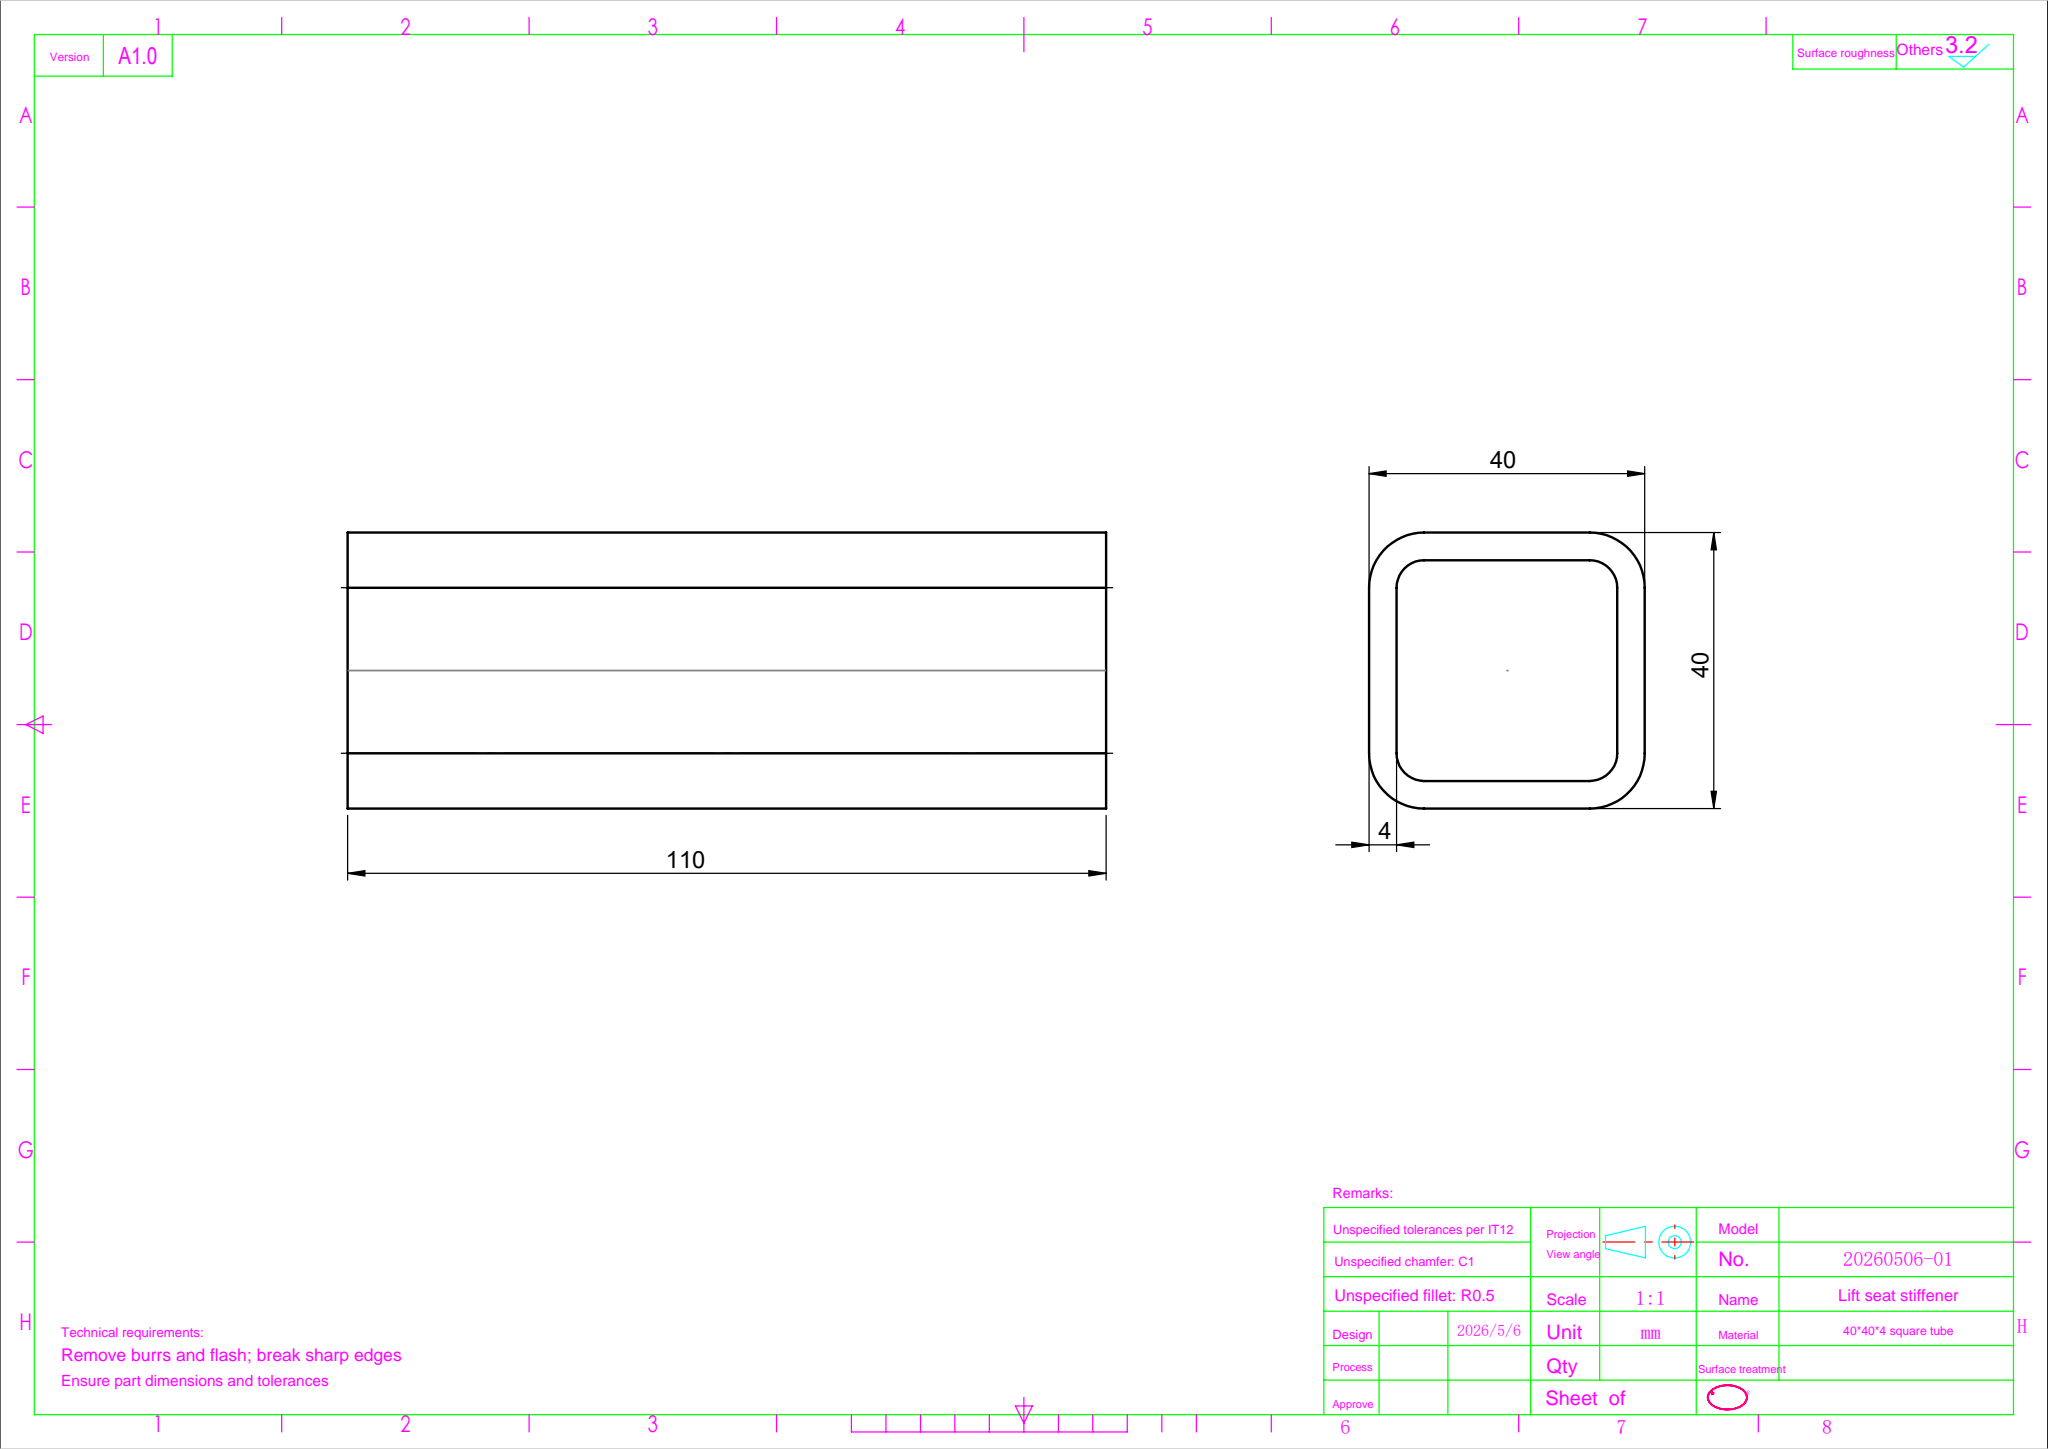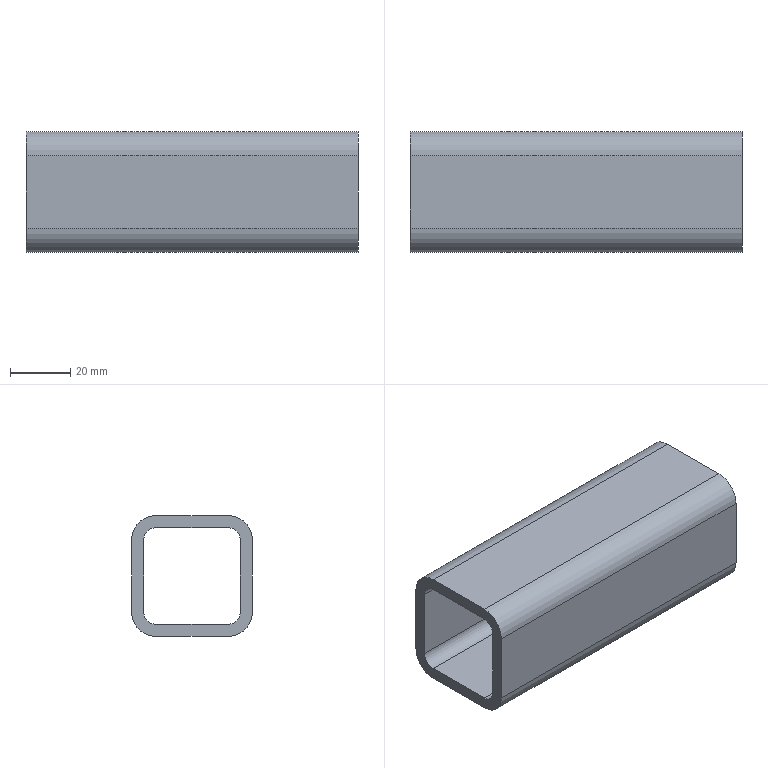Part | SolidWorks | features 3DProfileFeature 1, WeldMemberFeat 1, WeldmentFeature 1 | 1 solid | 18 faces | box 110 x 40 x 40 mm | volume 58828 mm3 | plane 10 | cylinder 8 | commonest cylinder face diameters 8 x4 16 x4
STEP:
#1=CARTESIAN_POINT('',(0.,12.,-20.));
#2=VERTEX_POINT('',#1);
#3=CARTESIAN_POINT('',(0.,20.,-12.));
#4=VERTEX_POINT('',#3);
#5=CARTESIAN_POINT('',(0.,12.,-12.));
#6=DIRECTION('',(1.,0.,0.));
#7=DIRECTION('',(0.,0.,-1.));
#8=AXIS2_PLACEMENT_3D('',#5,#6,#7);
#9=CIRCLE('',#8,8.);
#10=EDGE_CURVE('',#2,#4,#9,.T.);
#11=ORIENTED_EDGE('',*,*,#10,.T.);
#12=CARTESIAN_POINT('',(110.,20.,-12.));
#13=VERTEX_POINT('',#12);
#14=CARTESIAN_POINT('',(110.,20.,-12.));
#15=DIRECTION('',(-1.,0.,0.));
#16=VECTOR('',#15,1000.);
#17=LINE('',#14,#16);
#18=EDGE_CURVE('',#13,#4,#17,.T.);
#19=ORIENTED_EDGE('',*,*,#18,.F.);
#20=CARTESIAN_POINT('',(110.,12.,-20.));
#21=VERTEX_POINT('',#20);
#22=CARTESIAN_POINT('',(110.,12.,-12.));
#23=DIRECTION('',(1.,0.,0.));
#24=DIRECTION('',(0.,0.,-1.));
#25=AXIS2_PLACEMENT_3D('',#22,#23,#24);
#26=CIRCLE('',#25,8.);
#27=EDGE_CURVE('',#21,#13,#26,.T.);
#28=ORIENTED_EDGE('',*,*,#27,.F.);
#29=CARTESIAN_POINT('',(110.,12.,-20.));
#30=DIRECTION('',(-1.,0.,0.));
#31=VECTOR('',#30,1000.);
#32=LINE('',#29,#31);
#33=EDGE_CURVE('',#21,#2,#32,.T.);
#34=ORIENTED_EDGE('',*,*,#33,.T.);
#35=EDGE_LOOP('',(#11,#19,#28,#34));
#36=FACE_OUTER_BOUND('',#35,.T.);
#37=CARTESIAN_POINT('',(110.,12.,-12.));
#38=DIRECTION('',(-1.,0.,0.));
#39=DIRECTION('',(0.,0.,1.));
#40=AXIS2_PLACEMENT_3D('',#37,#38,#39);
#41=CYLINDRICAL_SURFACE('',#40,8.);
#42=ADVANCED_FACE('',(#36),#41,.T.);
#43=CARTESIAN_POINT('',(0.,20.,12.));
#44=VERTEX_POINT('',#43);
#45=CARTESIAN_POINT('',(0.,20.,-12.));
#46=DIRECTION('',(0.,0.,1.));
#47=VECTOR('',#46,1000.);
#48=LINE('',#45,#47);
#49=EDGE_CURVE('',#4,#44,#48,.T.);
#50=ORIENTED_EDGE('',*,*,#49,.T.);
#51=CARTESIAN_POINT('',(110.,20.,12.));
#52=VERTEX_POINT('',#51);
#53=CARTESIAN_POINT('',(110.,20.,12.));
#54=DIRECTION('',(-1.,0.,0.));
#55=VECTOR('',#54,1000.);
#56=LINE('',#53,#55);
#57=EDGE_CURVE('',#52,#44,#56,.T.);
#58=ORIENTED_EDGE('',*,*,#57,.F.);
#59=CARTESIAN_POINT('',(110.,20.,-12.));
#60=DIRECTION('',(0.,0.,1.));
#61=VECTOR('',#60,1000.);
#62=LINE('',#59,#61);
#63=EDGE_CURVE('',#13,#52,#62,.T.);
#64=ORIENTED_EDGE('',*,*,#63,.F.);
#65=ORIENTED_EDGE('',*,*,#18,.T.);
#66=EDGE_LOOP('',(#50,#58,#64,#65));
#67=FACE_OUTER_BOUND('',#66,.T.);
#68=CARTESIAN_POINT('',(110.,20.,-12.));
#69=DIRECTION('',(0.,-1.,0.));
#70=DIRECTION('',(0.,0.,-1.));
#71=AXIS2_PLACEMENT_3D('',#68,#69,#70);
#72=PLANE('',#71);
#73=ADVANCED_FACE('',(#67),#72,.F.);
#74=CARTESIAN_POINT('',(0.,12.,20.));
#75=VERTEX_POINT('',#74);
#76=CARTESIAN_POINT('',(0.,12.,12.));
#77=DIRECTION('',(1.,0.,0.));
#78=DIRECTION('',(0.,0.,-1.));
#79=AXIS2_PLACEMENT_3D('',#76,#77,#78);
#80=CIRCLE('',#79,8.);
#81=EDGE_CURVE('',#44,#75,#80,.T.);
#82=ORIENTED_EDGE('',*,*,#81,.T.);
#83=CARTESIAN_POINT('',(110.,12.,20.));
#84=VERTEX_POINT('',#83);
#85=CARTESIAN_POINT('',(110.,12.,20.));
#86=DIRECTION('',(-1.,0.,0.));
#87=VECTOR('',#86,1000.);
#88=LINE('',#85,#87);
#89=EDGE_CURVE('',#84,#75,#88,.T.);
#90=ORIENTED_EDGE('',*,*,#89,.F.);
#91=CARTESIAN_POINT('',(110.,12.,12.));
#92=DIRECTION('',(1.,0.,0.));
#93=DIRECTION('',(0.,0.,-1.));
#94=AXIS2_PLACEMENT_3D('',#91,#92,#93);
#95=CIRCLE('',#94,8.);
#96=EDGE_CURVE('',#52,#84,#95,.T.);
#97=ORIENTED_EDGE('',*,*,#96,.F.);
#98=ORIENTED_EDGE('',*,*,#57,.T.);
#99=EDGE_LOOP('',(#82,#90,#97,#98));
#100=FACE_OUTER_BOUND('',#99,.T.);
#101=CARTESIAN_POINT('',(110.,12.,12.));
#102=DIRECTION('',(-1.,0.,0.));
#103=DIRECTION('',(0.,0.,1.));
#104=AXIS2_PLACEMENT_3D('',#101,#102,#103);
#105=CYLINDRICAL_SURFACE('',#104,8.);
#106=ADVANCED_FACE('',(#100),#105,.T.);
#107=CARTESIAN_POINT('',(0.,-12.,20.));
#108=VERTEX_POINT('',#107);
#109=CARTESIAN_POINT('',(0.,-12.,20.));
#110=DIRECTION('',(0.,-1.,0.));
#111=VECTOR('',#110,1000.);
#112=LINE('',#109,#111);
#113=EDGE_CURVE('',#75,#108,#112,.T.);
#114=ORIENTED_EDGE('',*,*,#113,.T.);
#115=CARTESIAN_POINT('',(110.,-12.,20.));
#116=VERTEX_POINT('',#115);
#117=CARTESIAN_POINT('',(110.,-12.,20.));
#118=DIRECTION('',(-1.,0.,0.));
#119=VECTOR('',#118,1000.);
#120=LINE('',#117,#119);
#121=EDGE_CURVE('',#116,#108,#120,.T.);
#122=ORIENTED_EDGE('',*,*,#121,.F.);
#123=CARTESIAN_POINT('',(110.,-12.,20.));
#124=DIRECTION('',(0.,-1.,0.));
#125=VECTOR('',#124,1000.);
#126=LINE('',#123,#125);
#127=EDGE_CURVE('',#84,#116,#126,.T.);
#128=ORIENTED_EDGE('',*,*,#127,.F.);
#129=ORIENTED_EDGE('',*,*,#89,.T.);
#130=EDGE_LOOP('',(#114,#122,#128,#129));
#131=FACE_OUTER_BOUND('',#130,.T.);
#132=CARTESIAN_POINT('',(110.,-12.,20.));
#133=DIRECTION('',(0.,0.,-1.));
#134=DIRECTION('',(-1.,0.,0.));
#135=AXIS2_PLACEMENT_3D('',#132,#133,#134);
#136=PLANE('',#135);
#137=ADVANCED_FACE('',(#131),#136,.F.);
#138=CARTESIAN_POINT('',(0.,-20.,12.));
#139=VERTEX_POINT('',#138);
#140=CARTESIAN_POINT('',(0.,-12.,12.));
#141=DIRECTION('',(1.,0.,0.));
#142=DIRECTION('',(0.,0.,-1.));
#143=AXIS2_PLACEMENT_3D('',#140,#141,#142);
#144=CIRCLE('',#143,8.);
#145=EDGE_CURVE('',#108,#139,#144,.T.);
#146=ORIENTED_EDGE('',*,*,#145,.T.);
#147=CARTESIAN_POINT('',(110.,-20.,12.));
#148=VERTEX_POINT('',#147);
#149=CARTESIAN_POINT('',(110.,-20.,12.));
#150=DIRECTION('',(-1.,0.,0.));
#151=VECTOR('',#150,1000.);
#152=LINE('',#149,#151);
#153=EDGE_CURVE('',#148,#139,#152,.T.);
#154=ORIENTED_EDGE('',*,*,#153,.F.);
#155=CARTESIAN_POINT('',(110.,-12.,12.));
#156=DIRECTION('',(1.,0.,0.));
#157=DIRECTION('',(0.,0.,-1.));
#158=AXIS2_PLACEMENT_3D('',#155,#156,#157);
#159=CIRCLE('',#158,8.);
#160=EDGE_CURVE('',#116,#148,#159,.T.);
#161=ORIENTED_EDGE('',*,*,#160,.F.);
#162=ORIENTED_EDGE('',*,*,#121,.T.);
#163=EDGE_LOOP('',(#146,#154,#161,#162));
#164=FACE_OUTER_BOUND('',#163,.T.);
#165=CARTESIAN_POINT('',(110.,-12.,12.));
#166=DIRECTION('',(-1.,0.,0.));
#167=DIRECTION('',(0.,0.,1.));
#168=AXIS2_PLACEMENT_3D('',#165,#166,#167);
#169=CYLINDRICAL_SURFACE('',#168,8.);
#170=ADVANCED_FACE('',(#164),#169,.T.);
#171=CARTESIAN_POINT('',(0.,-20.,-12.));
#172=VERTEX_POINT('',#171);
#173=CARTESIAN_POINT('',(0.,-20.,12.));
#174=DIRECTION('',(0.,0.,-1.));
#175=VECTOR('',#174,1000.);
#176=LINE('',#173,#175);
#177=EDGE_CURVE('',#139,#172,#176,.T.);
#178=ORIENTED_EDGE('',*,*,#177,.T.);
#179=CARTESIAN_POINT('',(110.,-20.,-12.));
#180=VERTEX_POINT('',#179);
#181=CARTESIAN_POINT('',(110.,-20.,-12.));
#182=DIRECTION('',(-1.,0.,0.));
#183=VECTOR('',#182,1000.);
#184=LINE('',#181,#183);
#185=EDGE_CURVE('',#180,#172,#184,.T.);
#186=ORIENTED_EDGE('',*,*,#185,.F.);
#187=CARTESIAN_POINT('',(110.,-20.,12.));
#188=DIRECTION('',(0.,0.,-1.));
#189=VECTOR('',#188,1000.);
#190=LINE('',#187,#189);
#191=EDGE_CURVE('',#148,#180,#190,.T.);
#192=ORIENTED_EDGE('',*,*,#191,.F.);
#193=ORIENTED_EDGE('',*,*,#153,.T.);
#194=EDGE_LOOP('',(#178,#186,#192,#193));
#195=FACE_OUTER_BOUND('',#194,.T.);
#196=CARTESIAN_POINT('',(110.,-20.,12.));
#197=DIRECTION('',(0.,1.,0.));
#198=DIRECTION('',(0.,0.,1.));
#199=AXIS2_PLACEMENT_3D('',#196,#197,#198);
#200=PLANE('',#199);
#201=ADVANCED_FACE('',(#195),#200,.F.);
#202=CARTESIAN_POINT('',(0.,-12.,-20.));
#203=VERTEX_POINT('',#202);
#204=CARTESIAN_POINT('',(0.,-12.,-12.));
#205=DIRECTION('',(1.,0.,0.));
#206=DIRECTION('',(0.,0.,-1.));
#207=AXIS2_PLACEMENT_3D('',#204,#205,#206);
#208=CIRCLE('',#207,8.);
#209=EDGE_CURVE('',#172,#203,#208,.T.);
#210=ORIENTED_EDGE('',*,*,#209,.T.);
#211=CARTESIAN_POINT('',(110.,-12.,-20.));
#212=VERTEX_POINT('',#211);
#213=CARTESIAN_POINT('',(110.,-12.,-20.));
#214=DIRECTION('',(-1.,0.,0.));
#215=VECTOR('',#214,1000.);
#216=LINE('',#213,#215);
#217=EDGE_CURVE('',#212,#203,#216,.T.);
#218=ORIENTED_EDGE('',*,*,#217,.F.);
#219=CARTESIAN_POINT('',(110.,-12.,-12.));
#220=DIRECTION('',(1.,0.,0.));
#221=DIRECTION('',(0.,0.,-1.));
#222=AXIS2_PLACEMENT_3D('',#219,#220,#221);
#223=CIRCLE('',#222,8.);
#224=EDGE_CURVE('',#180,#212,#223,.T.);
#225=ORIENTED_EDGE('',*,*,#224,.F.);
#226=ORIENTED_EDGE('',*,*,#185,.T.);
#227=EDGE_LOOP('',(#210,#218,#225,#226));
#228=FACE_OUTER_BOUND('',#227,.T.);
#229=CARTESIAN_POINT('',(110.,-12.,-12.));
#230=DIRECTION('',(-1.,0.,0.));
#231=DIRECTION('',(0.,0.,1.));
#232=AXIS2_PLACEMENT_3D('',#229,#230,#231);
#233=CYLINDRICAL_SURFACE('',#232,8.);
#234=ADVANCED_FACE('',(#228),#233,.T.);
#235=CARTESIAN_POINT('',(0.,16.,12.));
#236=VERTEX_POINT('',#235);
#237=CARTESIAN_POINT('',(0.,12.,16.));
#238=VERTEX_POINT('',#237);
#239=CARTESIAN_POINT('',(0.,12.,12.));
#240=DIRECTION('',(1.,0.,0.));
#241=DIRECTION('',(0.,0.,-1.));
#242=AXIS2_PLACEMENT_3D('',#239,#240,#241);
#243=CIRCLE('',#242,4.);
#244=EDGE_CURVE('',#236,#238,#243,.T.);
#245=ORIENTED_EDGE('',*,*,#244,.F.);
#246=CARTESIAN_POINT('',(110.,16.,12.));
#247=VERTEX_POINT('',#246);
#248=CARTESIAN_POINT('',(110.,16.,12.));
#249=DIRECTION('',(-1.,0.,0.));
#250=VECTOR('',#249,1000.);
#251=LINE('',#248,#250);
#252=EDGE_CURVE('',#247,#236,#251,.T.);
#253=ORIENTED_EDGE('',*,*,#252,.F.);
#254=CARTESIAN_POINT('',(110.,12.,16.));
#255=VERTEX_POINT('',#254);
#256=CARTESIAN_POINT('',(110.,12.,12.));
#257=DIRECTION('',(1.,0.,0.));
#258=DIRECTION('',(0.,0.,-1.));
#259=AXIS2_PLACEMENT_3D('',#256,#257,#258);
#260=CIRCLE('',#259,4.);
#261=EDGE_CURVE('',#247,#255,#260,.T.);
#262=ORIENTED_EDGE('',*,*,#261,.T.);
#263=CARTESIAN_POINT('',(110.,12.,16.));
#264=DIRECTION('',(-1.,0.,0.));
#265=VECTOR('',#264,1000.);
#266=LINE('',#263,#265);
#267=EDGE_CURVE('',#255,#238,#266,.T.);
#268=ORIENTED_EDGE('',*,*,#267,.T.);
#269=EDGE_LOOP('',(#245,#253,#262,#268));
#270=FACE_OUTER_BOUND('',#269,.T.);
#271=CARTESIAN_POINT('',(110.,12.,12.));
#272=DIRECTION('',(-1.,0.,0.));
#273=DIRECTION('',(0.,0.,1.));
#274=AXIS2_PLACEMENT_3D('',#271,#272,#273);
#275=CYLINDRICAL_SURFACE('',#274,4.);
#276=ADVANCED_FACE('',(#270),#275,.F.);
#277=CARTESIAN_POINT('',(0.,16.,-12.));
#278=VERTEX_POINT('',#277);
#279=CARTESIAN_POINT('',(0.,16.,-12.));
#280=DIRECTION('',(0.,0.,1.));
#281=VECTOR('',#280,1000.);
#282=LINE('',#279,#281);
#283=EDGE_CURVE('',#278,#236,#282,.T.);
#284=ORIENTED_EDGE('',*,*,#283,.F.);
#285=CARTESIAN_POINT('',(110.,16.,-12.));
#286=VERTEX_POINT('',#285);
#287=CARTESIAN_POINT('',(110.,16.,-12.));
#288=DIRECTION('',(-1.,0.,0.));
#289=VECTOR('',#288,1000.);
#290=LINE('',#287,#289);
#291=EDGE_CURVE('',#286,#278,#290,.T.);
#292=ORIENTED_EDGE('',*,*,#291,.F.);
#293=CARTESIAN_POINT('',(110.,16.,-12.));
#294=DIRECTION('',(0.,0.,1.));
#295=VECTOR('',#294,1000.);
#296=LINE('',#293,#295);
#297=EDGE_CURVE('',#286,#247,#296,.T.);
#298=ORIENTED_EDGE('',*,*,#297,.T.);
#299=ORIENTED_EDGE('',*,*,#252,.T.);
#300=EDGE_LOOP('',(#284,#292,#298,#299));
#301=FACE_OUTER_BOUND('',#300,.T.);
#302=CARTESIAN_POINT('',(110.,16.,-12.));
#303=DIRECTION('',(0.,-1.,0.));
#304=DIRECTION('',(0.,0.,-1.));
#305=AXIS2_PLACEMENT_3D('',#302,#303,#304);
#306=PLANE('',#305);
#307=ADVANCED_FACE('',(#301),#306,.T.);
#308=CARTESIAN_POINT('',(0.,12.,-16.));
#309=VERTEX_POINT('',#308);
#310=CARTESIAN_POINT('',(0.,12.,-12.));
#311=DIRECTION('',(1.,0.,0.));
#312=DIRECTION('',(0.,0.,-1.));
#313=AXIS2_PLACEMENT_3D('',#310,#311,#312);
#314=CIRCLE('',#313,4.);
#315=EDGE_CURVE('',#309,#278,#314,.T.);
#316=ORIENTED_EDGE('',*,*,#315,.F.);
#317=CARTESIAN_POINT('',(110.,12.,-16.));
#318=VERTEX_POINT('',#317);
#319=CARTESIAN_POINT('',(110.,12.,-16.));
#320=DIRECTION('',(-1.,0.,0.));
#321=VECTOR('',#320,1000.);
#322=LINE('',#319,#321);
#323=EDGE_CURVE('',#318,#309,#322,.T.);
#324=ORIENTED_EDGE('',*,*,#323,.F.);
#325=CARTESIAN_POINT('',(110.,12.,-12.));
#326=DIRECTION('',(1.,0.,0.));
#327=DIRECTION('',(0.,0.,-1.));
#328=AXIS2_PLACEMENT_3D('',#325,#326,#327);
#329=CIRCLE('',#328,4.);
#330=EDGE_CURVE('',#318,#286,#329,.T.);
#331=ORIENTED_EDGE('',*,*,#330,.T.);
#332=ORIENTED_EDGE('',*,*,#291,.T.);
#333=EDGE_LOOP('',(#316,#324,#331,#332));
#334=FACE_OUTER_BOUND('',#333,.T.);
#335=CARTESIAN_POINT('',(110.,12.,-12.));
#336=DIRECTION('',(-1.,0.,0.));
#337=DIRECTION('',(0.,0.,1.));
#338=AXIS2_PLACEMENT_3D('',#335,#336,#337);
#339=CYLINDRICAL_SURFACE('',#338,4.);
#340=ADVANCED_FACE('',(#334),#339,.F.);
#341=CARTESIAN_POINT('',(0.,-12.,-16.));
#342=VERTEX_POINT('',#341);
#343=CARTESIAN_POINT('',(0.,12.,-16.));
#344=DIRECTION('',(0.,1.,0.));
#345=VECTOR('',#344,1000.);
#346=LINE('',#343,#345);
#347=EDGE_CURVE('',#342,#309,#346,.T.);
#348=ORIENTED_EDGE('',*,*,#347,.F.);
#349=CARTESIAN_POINT('',(110.,-12.,-16.));
#350=VERTEX_POINT('',#349);
#351=CARTESIAN_POINT('',(110.,-12.,-16.));
#352=DIRECTION('',(-1.,0.,0.));
#353=VECTOR('',#352,1000.);
#354=LINE('',#351,#353);
#355=EDGE_CURVE('',#350,#342,#354,.T.);
#356=ORIENTED_EDGE('',*,*,#355,.F.);
#357=CARTESIAN_POINT('',(110.,12.,-16.));
#358=DIRECTION('',(0.,1.,0.));
#359=VECTOR('',#358,1000.);
#360=LINE('',#357,#359);
#361=EDGE_CURVE('',#350,#318,#360,.T.);
#362=ORIENTED_EDGE('',*,*,#361,.T.);
#363=ORIENTED_EDGE('',*,*,#323,.T.);
#364=EDGE_LOOP('',(#348,#356,#362,#363));
#365=FACE_OUTER_BOUND('',#364,.T.);
#366=CARTESIAN_POINT('',(110.,12.,-16.));
#367=DIRECTION('',(0.,0.,1.));
#368=DIRECTION('',(1.,0.,0.));
#369=AXIS2_PLACEMENT_3D('',#366,#367,#368);
#370=PLANE('',#369);
#371=ADVANCED_FACE('',(#365),#370,.T.);
#372=CARTESIAN_POINT('',(0.,-16.,-12.));
#373=VERTEX_POINT('',#372);
#374=CARTESIAN_POINT('',(0.,-12.,-12.));
#375=DIRECTION('',(1.,0.,0.));
#376=DIRECTION('',(0.,0.,-1.));
#377=AXIS2_PLACEMENT_3D('',#374,#375,#376);
#378=CIRCLE('',#377,4.);
#379=EDGE_CURVE('',#373,#342,#378,.T.);
#380=ORIENTED_EDGE('',*,*,#379,.F.);
#381=CARTESIAN_POINT('',(110.,-16.,-12.));
#382=VERTEX_POINT('',#381);
#383=CARTESIAN_POINT('',(110.,-16.,-12.));
#384=DIRECTION('',(-1.,0.,0.));
#385=VECTOR('',#384,1000.);
#386=LINE('',#383,#385);
#387=EDGE_CURVE('',#382,#373,#386,.T.);
#388=ORIENTED_EDGE('',*,*,#387,.F.);
#389=CARTESIAN_POINT('',(110.,-12.,-12.));
#390=DIRECTION('',(1.,0.,0.));
#391=DIRECTION('',(0.,0.,-1.));
#392=AXIS2_PLACEMENT_3D('',#389,#390,#391);
#393=CIRCLE('',#392,4.);
#394=EDGE_CURVE('',#382,#350,#393,.T.);
#395=ORIENTED_EDGE('',*,*,#394,.T.);
#396=ORIENTED_EDGE('',*,*,#355,.T.);
#397=EDGE_LOOP('',(#380,#388,#395,#396));
#398=FACE_OUTER_BOUND('',#397,.T.);
#399=CARTESIAN_POINT('',(110.,-12.,-12.));
#400=DIRECTION('',(-1.,0.,0.));
#401=DIRECTION('',(0.,0.,1.));
#402=AXIS2_PLACEMENT_3D('',#399,#400,#401);
#403=CYLINDRICAL_SURFACE('',#402,4.);
#404=ADVANCED_FACE('',(#398),#403,.F.);
#405=CARTESIAN_POINT('',(0.,-16.,12.));
#406=VERTEX_POINT('',#405);
#407=CARTESIAN_POINT('',(0.,-16.,12.));
#408=DIRECTION('',(0.,0.,-1.));
#409=VECTOR('',#408,1000.);
#410=LINE('',#407,#409);
#411=EDGE_CURVE('',#406,#373,#410,.T.);
#412=ORIENTED_EDGE('',*,*,#411,.F.);
#413=CARTESIAN_POINT('',(110.,-16.,12.));
#414=VERTEX_POINT('',#413);
#415=CARTESIAN_POINT('',(110.,-16.,12.));
#416=DIRECTION('',(-1.,0.,0.));
#417=VECTOR('',#416,1000.);
#418=LINE('',#415,#417);
#419=EDGE_CURVE('',#414,#406,#418,.T.);
#420=ORIENTED_EDGE('',*,*,#419,.F.);
#421=CARTESIAN_POINT('',(110.,-16.,12.));
#422=DIRECTION('',(0.,0.,-1.));
#423=VECTOR('',#422,1000.);
#424=LINE('',#421,#423);
#425=EDGE_CURVE('',#414,#382,#424,.T.);
#426=ORIENTED_EDGE('',*,*,#425,.T.);
#427=ORIENTED_EDGE('',*,*,#387,.T.);
#428=EDGE_LOOP('',(#412,#420,#426,#427));
#429=FACE_OUTER_BOUND('',#428,.T.);
#430=CARTESIAN_POINT('',(110.,-16.,12.));
#431=DIRECTION('',(0.,1.,0.));
#432=DIRECTION('',(0.,0.,1.));
#433=AXIS2_PLACEMENT_3D('',#430,#431,#432);
#434=PLANE('',#433);
#435=ADVANCED_FACE('',(#429),#434,.T.);
#436=CARTESIAN_POINT('',(0.,-12.,16.));
#437=VERTEX_POINT('',#436);
#438=CARTESIAN_POINT('',(0.,-12.,12.));
#439=DIRECTION('',(1.,0.,0.));
#440=DIRECTION('',(0.,0.,-1.));
#441=AXIS2_PLACEMENT_3D('',#438,#439,#440);
#442=CIRCLE('',#441,4.);
#443=EDGE_CURVE('',#437,#406,#442,.T.);
#444=ORIENTED_EDGE('',*,*,#443,.F.);
#445=CARTESIAN_POINT('',(110.,-12.,16.));
#446=VERTEX_POINT('',#445);
#447=CARTESIAN_POINT('',(110.,-12.,16.));
#448=DIRECTION('',(-1.,0.,0.));
#449=VECTOR('',#448,1000.);
#450=LINE('',#447,#449);
#451=EDGE_CURVE('',#446,#437,#450,.T.);
#452=ORIENTED_EDGE('',*,*,#451,.F.);
#453=CARTESIAN_POINT('',(110.,-12.,12.));
#454=DIRECTION('',(1.,0.,0.));
#455=DIRECTION('',(0.,0.,-1.));
#456=AXIS2_PLACEMENT_3D('',#453,#454,#455);
#457=CIRCLE('',#456,4.);
#458=EDGE_CURVE('',#446,#414,#457,.T.);
#459=ORIENTED_EDGE('',*,*,#458,.T.);
#460=ORIENTED_EDGE('',*,*,#419,.T.);
#461=EDGE_LOOP('',(#444,#452,#459,#460));
#462=FACE_OUTER_BOUND('',#461,.T.);
#463=CARTESIAN_POINT('',(110.,-12.,12.));
#464=DIRECTION('',(-1.,0.,0.));
#465=DIRECTION('',(0.,0.,1.));
#466=AXIS2_PLACEMENT_3D('',#463,#464,#465);
#467=CYLINDRICAL_SURFACE('',#466,4.);
#468=ADVANCED_FACE('',(#462),#467,.F.);
#469=CARTESIAN_POINT('',(0.,-12.,16.));
#470=DIRECTION('',(0.,-1.,0.));
#471=VECTOR('',#470,1000.);
#472=LINE('',#469,#471);
#473=EDGE_CURVE('',#238,#437,#472,.T.);
#474=ORIENTED_EDGE('',*,*,#473,.F.);
#475=ORIENTED_EDGE('',*,*,#267,.F.);
#476=CARTESIAN_POINT('',(110.,-12.,16.));
#477=DIRECTION('',(0.,-1.,0.));
#478=VECTOR('',#477,1000.);
#479=LINE('',#476,#478);
#480=EDGE_CURVE('',#255,#446,#479,.T.);
#481=ORIENTED_EDGE('',*,*,#480,.T.);
#482=ORIENTED_EDGE('',*,*,#451,.T.);
#483=EDGE_LOOP('',(#474,#475,#481,#482));
#484=FACE_OUTER_BOUND('',#483,.T.);
#485=CARTESIAN_POINT('',(110.,-12.,16.));
#486=DIRECTION('',(0.,0.,-1.));
#487=DIRECTION('',(-1.,0.,0.));
#488=AXIS2_PLACEMENT_3D('',#485,#486,#487);
#489=PLANE('',#488);
#490=ADVANCED_FACE('',(#484),#489,.T.);
#491=CARTESIAN_POINT('',(0.,12.,-20.));
#492=DIRECTION('',(0.,1.,0.));
#493=VECTOR('',#492,1000.);
#494=LINE('',#491,#493);
#495=EDGE_CURVE('',#203,#2,#494,.T.);
#496=ORIENTED_EDGE('',*,*,#495,.T.);
#497=ORIENTED_EDGE('',*,*,#33,.F.);
#498=CARTESIAN_POINT('',(110.,12.,-20.));
#499=DIRECTION('',(0.,1.,0.));
#500=VECTOR('',#499,1000.);
#501=LINE('',#498,#500);
#502=EDGE_CURVE('',#212,#21,#501,.T.);
#503=ORIENTED_EDGE('',*,*,#502,.F.);
#504=ORIENTED_EDGE('',*,*,#217,.T.);
#505=EDGE_LOOP('',(#496,#497,#503,#504));
#506=FACE_OUTER_BOUND('',#505,.T.);
#507=CARTESIAN_POINT('',(110.,12.,-20.));
#508=DIRECTION('',(0.,0.,1.));
#509=DIRECTION('',(1.,0.,0.));
#510=AXIS2_PLACEMENT_3D('',#507,#508,#509);
#511=PLANE('',#510);
#512=ADVANCED_FACE('',(#506),#511,.F.);
#513=ORIENTED_EDGE('',*,*,#261,.F.);
#514=ORIENTED_EDGE('',*,*,#297,.F.);
#515=ORIENTED_EDGE('',*,*,#330,.F.);
#516=ORIENTED_EDGE('',*,*,#361,.F.);
#517=ORIENTED_EDGE('',*,*,#394,.F.);
#518=ORIENTED_EDGE('',*,*,#425,.F.);
#519=ORIENTED_EDGE('',*,*,#458,.F.);
#520=ORIENTED_EDGE('',*,*,#480,.F.);
#521=EDGE_LOOP('',(#513,#514,#515,#516,#517,#518,#519,#520));
#522=FACE_BOUND('',#521,.T.);
#523=ORIENTED_EDGE('',*,*,#27,.T.);
#524=ORIENTED_EDGE('',*,*,#63,.T.);
#525=ORIENTED_EDGE('',*,*,#96,.T.);
#526=ORIENTED_EDGE('',*,*,#127,.T.);
#527=ORIENTED_EDGE('',*,*,#160,.T.);
#528=ORIENTED_EDGE('',*,*,#191,.T.);
#529=ORIENTED_EDGE('',*,*,#224,.T.);
#530=ORIENTED_EDGE('',*,*,#502,.T.);
#531=EDGE_LOOP('',(#523,#524,#525,#526,#527,#528,#529,#530));
#532=FACE_OUTER_BOUND('',#531,.T.);
#533=CARTESIAN_POINT('',(110.,12.,-12.));
#534=DIRECTION('',(1.,0.,0.));
#535=DIRECTION('',(0.,0.,-1.));
#536=AXIS2_PLACEMENT_3D('',#533,#534,#535);
#537=PLANE('',#536);
#538=ADVANCED_FACE('',(#522,#532),#537,.T.);
#539=ORIENTED_EDGE('',*,*,#244,.T.);
#540=ORIENTED_EDGE('',*,*,#473,.T.);
#541=ORIENTED_EDGE('',*,*,#443,.T.);
#542=ORIENTED_EDGE('',*,*,#411,.T.);
#543=ORIENTED_EDGE('',*,*,#379,.T.);
#544=ORIENTED_EDGE('',*,*,#347,.T.);
#545=ORIENTED_EDGE('',*,*,#315,.T.);
#546=ORIENTED_EDGE('',*,*,#283,.T.);
#547=EDGE_LOOP('',(#539,#540,#541,#542,#543,#544,#545,#546));
#548=FACE_BOUND('',#547,.T.);
#549=ORIENTED_EDGE('',*,*,#10,.F.);
#550=ORIENTED_EDGE('',*,*,#495,.F.);
#551=ORIENTED_EDGE('',*,*,#209,.F.);
#552=ORIENTED_EDGE('',*,*,#177,.F.);
#553=ORIENTED_EDGE('',*,*,#145,.F.);
#554=ORIENTED_EDGE('',*,*,#113,.F.);
#555=ORIENTED_EDGE('',*,*,#81,.F.);
#556=ORIENTED_EDGE('',*,*,#49,.F.);
#557=EDGE_LOOP('',(#549,#550,#551,#552,#553,#554,#555,#556));
#558=FACE_OUTER_BOUND('',#557,.T.);
#559=CARTESIAN_POINT('',(0.,12.,-12.));
#560=DIRECTION('',(1.,0.,0.));
#561=DIRECTION('',(0.,0.,-1.));
#562=AXIS2_PLACEMENT_3D('',#559,#560,#561);
#563=PLANE('',#562);
#564=ADVANCED_FACE('',(#548,#558),#563,.F.);
#565=CLOSED_SHELL('',(#42,#73,#106,#137,#170,#201,#234,#276,#307,#340,#371,#404,#435,#468,#490,#512,#538,#564));
#566=MANIFOLD_SOLID_BREP('',#565);
#567=CARTESIAN_POINT('',(0.,0.,0.));
#568=DIRECTION('',(0.,0.,1.));
#569=DIRECTION('',(1.,0.,0.));
#570=AXIS2_PLACEMENT_3D('',#567,#568,#569);
#571=(LENGTH_UNIT()NAMED_UNIT(*)SI_UNIT(.MILLI.,.METRE.));
#572=UNCERTAINTY_MEASURE_WITH_UNIT(LENGTH_MEASURE(0.00001),#571,'','');
#573=(NAMED_UNIT(*)PLANE_ANGLE_UNIT()SI_UNIT($,.RADIAN.));
#574=(NAMED_UNIT(*)SI_UNIT($,.STERADIAN.)SOLID_ANGLE_UNIT());
#575=(GEOMETRIC_REPRESENTATION_CONTEXT(3)GLOBAL_UNCERTAINTY_ASSIGNED_CONTEXT((#572))GLOBAL_UNIT_ASSIGNED_CONTEXT((#571,#573,#574))REPRESENTATION_CONTEXT('',''));
#576=ADVANCED_BREP_SHAPE_REPRESENTATION('',(#566,#570),#575);